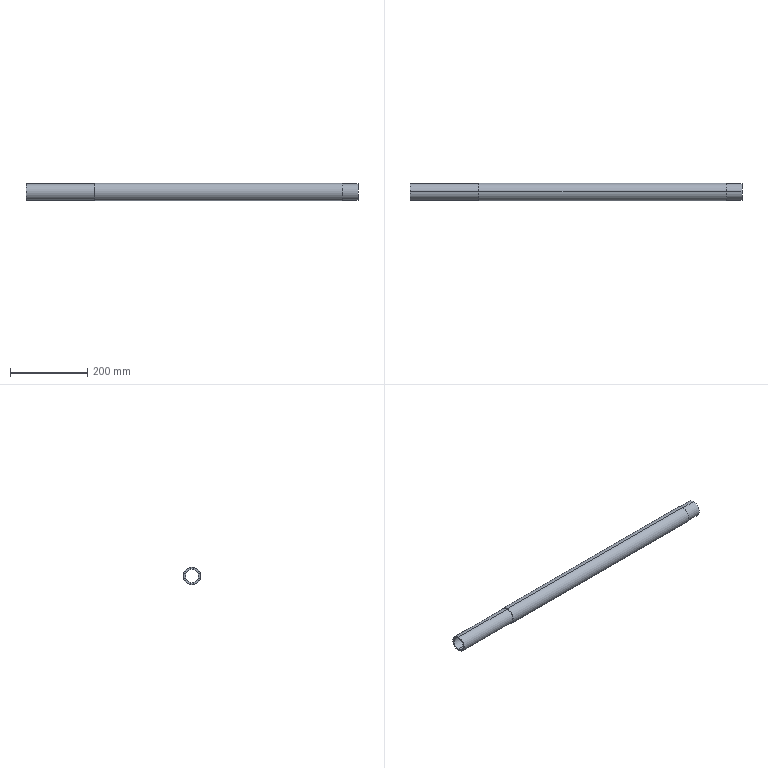Part | SolidWorks | features BaseBody 1 | 1 solid | 12 faces | box 860 x 45 x 45 mm | volume 542272 mm3 | cylinder 8 | plane 4 | commonest cylinder face diameters 42 x4 34 x2 45 x2
STEP:
#1=CARTESIAN_POINT('',(-430.,0.,17.));
#2=VERTEX_POINT('',#1);
#3=CARTESIAN_POINT('',(-430.,0.,-17.));
#4=VERTEX_POINT('',#3);
#5=CARTESIAN_POINT('',(-430.,0.,0.));
#6=DIRECTION('',(1.,0.,0.));
#7=DIRECTION('',(0.,0.,-1.));
#8=AXIS2_PLACEMENT_3D('',#5,#6,#7);
#9=CIRCLE('',#8,17.);
#10=EDGE_CURVE('',#2,#4,#9,.T.);
#11=ORIENTED_EDGE('',*,*,#10,.F.);
#12=CARTESIAN_POINT('',(430.,0.,17.));
#13=VERTEX_POINT('',#12);
#14=CARTESIAN_POINT('',(-473.,0.,17.));
#15=DIRECTION('',(1.,0.,0.));
#16=VECTOR('',#15,1000.);
#17=LINE('',#14,#16);
#18=EDGE_CURVE('',#2,#13,#17,.T.);
#19=ORIENTED_EDGE('',*,*,#18,.T.);
#20=CARTESIAN_POINT('',(430.,0.,-17.));
#21=VERTEX_POINT('',#20);
#22=CARTESIAN_POINT('',(430.,0.,0.));
#23=DIRECTION('',(-1.,0.,0.));
#24=DIRECTION('',(0.,0.,-1.));
#25=AXIS2_PLACEMENT_3D('',#22,#23,#24);
#26=CIRCLE('',#25,17.);
#27=EDGE_CURVE('',#21,#13,#26,.T.);
#28=ORIENTED_EDGE('',*,*,#27,.F.);
#29=CARTESIAN_POINT('',(-473.,0.,-17.));
#30=DIRECTION('',(1.,0.,0.));
#31=VECTOR('',#30,1000.);
#32=LINE('',#29,#31);
#33=EDGE_CURVE('',#4,#21,#32,.T.);
#34=ORIENTED_EDGE('',*,*,#33,.F.);
#35=EDGE_LOOP('',(#11,#19,#28,#34));
#36=FACE_OUTER_BOUND('',#35,.T.);
#37=CARTESIAN_POINT('',(-473.,0.,0.));
#38=DIRECTION('',(1.,0.,0.));
#39=DIRECTION('',(0.,0.,-1.));
#40=AXIS2_PLACEMENT_3D('',#37,#38,#39);
#41=CYLINDRICAL_SURFACE('',#40,17.);
#42=ADVANCED_FACE('',(#36),#41,.F.);
#43=CARTESIAN_POINT('',(390.,0.,-21.));
#44=VERTEX_POINT('',#43);
#45=CARTESIAN_POINT('',(390.,0.,21.));
#46=VERTEX_POINT('',#45);
#47=CARTESIAN_POINT('',(390.,0.,0.));
#48=DIRECTION('',(1.,0.,0.));
#49=DIRECTION('',(0.,0.,-1.));
#50=AXIS2_PLACEMENT_3D('',#47,#48,#49);
#51=CIRCLE('',#50,21.);
#52=EDGE_CURVE('',#44,#46,#51,.T.);
#53=ORIENTED_EDGE('',*,*,#52,.T.);
#54=CARTESIAN_POINT('',(430.,0.,21.));
#55=VERTEX_POINT('',#54);
#56=CARTESIAN_POINT('',(-473.,0.,21.));
#57=DIRECTION('',(1.,0.,0.));
#58=VECTOR('',#57,1000.);
#59=LINE('',#56,#58);
#60=EDGE_CURVE('',#46,#55,#59,.T.);
#61=ORIENTED_EDGE('',*,*,#60,.T.);
#62=CARTESIAN_POINT('',(430.,0.,-21.));
#63=VERTEX_POINT('',#62);
#64=CARTESIAN_POINT('',(430.,0.,0.));
#65=DIRECTION('',(1.,0.,0.));
#66=DIRECTION('',(0.,0.,-1.));
#67=AXIS2_PLACEMENT_3D('',#64,#65,#66);
#68=CIRCLE('',#67,21.);
#69=EDGE_CURVE('',#63,#55,#68,.T.);
#70=ORIENTED_EDGE('',*,*,#69,.F.);
#71=CARTESIAN_POINT('',(-473.,0.,-21.));
#72=DIRECTION('',(1.,0.,0.));
#73=VECTOR('',#72,1000.);
#74=LINE('',#71,#73);
#75=EDGE_CURVE('',#44,#63,#74,.T.);
#76=ORIENTED_EDGE('',*,*,#75,.F.);
#77=EDGE_LOOP('',(#53,#61,#70,#76));
#78=FACE_OUTER_BOUND('',#77,.T.);
#79=CARTESIAN_POINT('',(-473.,0.,0.));
#80=DIRECTION('',(1.,0.,0.));
#81=DIRECTION('',(0.,0.,-1.));
#82=AXIS2_PLACEMENT_3D('',#79,#80,#81);
#83=CYLINDRICAL_SURFACE('',#82,21.);
#84=ADVANCED_FACE('',(#78),#83,.T.);
#85=CARTESIAN_POINT('',(-430.,0.,-21.));
#86=VERTEX_POINT('',#85);
#87=CARTESIAN_POINT('',(-430.,0.,21.));
#88=VERTEX_POINT('',#87);
#89=CARTESIAN_POINT('',(-430.,0.,0.));
#90=DIRECTION('',(1.,0.,0.));
#91=DIRECTION('',(0.,0.,-1.));
#92=AXIS2_PLACEMENT_3D('',#89,#90,#91);
#93=CIRCLE('',#92,21.);
#94=EDGE_CURVE('',#86,#88,#93,.T.);
#95=ORIENTED_EDGE('',*,*,#94,.T.);
#96=CARTESIAN_POINT('',(-252.,0.,21.));
#97=VERTEX_POINT('',#96);
#98=CARTESIAN_POINT('',(-473.,0.,21.));
#99=DIRECTION('',(1.,0.,0.));
#100=VECTOR('',#99,1000.);
#101=LINE('',#98,#100);
#102=EDGE_CURVE('',#88,#97,#101,.T.);
#103=ORIENTED_EDGE('',*,*,#102,.T.);
#104=CARTESIAN_POINT('',(-252.,0.,-21.));
#105=VERTEX_POINT('',#104);
#106=CARTESIAN_POINT('',(-252.,0.,0.));
#107=DIRECTION('',(-1.,0.,0.));
#108=DIRECTION('',(0.,0.,-1.));
#109=AXIS2_PLACEMENT_3D('',#106,#107,#108);
#110=CIRCLE('',#109,21.);
#111=EDGE_CURVE('',#97,#105,#110,.T.);
#112=ORIENTED_EDGE('',*,*,#111,.T.);
#113=CARTESIAN_POINT('',(-473.,0.,-21.));
#114=DIRECTION('',(1.,0.,0.));
#115=VECTOR('',#114,1000.);
#116=LINE('',#113,#115);
#117=EDGE_CURVE('',#86,#105,#116,.T.);
#118=ORIENTED_EDGE('',*,*,#117,.F.);
#119=EDGE_LOOP('',(#95,#103,#112,#118));
#120=FACE_OUTER_BOUND('',#119,.T.);
#121=CARTESIAN_POINT('',(-473.,0.,0.));
#122=DIRECTION('',(1.,0.,0.));
#123=DIRECTION('',(0.,0.,-1.));
#124=AXIS2_PLACEMENT_3D('',#121,#122,#123);
#125=CYLINDRICAL_SURFACE('',#124,21.);
#126=ADVANCED_FACE('',(#120),#125,.T.);
#127=CARTESIAN_POINT('',(-252.,0.,-22.5));
#128=VERTEX_POINT('',#127);
#129=CARTESIAN_POINT('',(-252.,0.,22.5));
#130=VERTEX_POINT('',#129);
#131=CARTESIAN_POINT('',(-252.,0.,0.));
#132=DIRECTION('',(1.,0.,0.));
#133=DIRECTION('',(0.,0.,-1.));
#134=AXIS2_PLACEMENT_3D('',#131,#132,#133);
#135=CIRCLE('',#134,22.5);
#136=EDGE_CURVE('',#128,#130,#135,.T.);
#137=ORIENTED_EDGE('',*,*,#136,.T.);
#138=CARTESIAN_POINT('',(390.,0.,22.5));
#139=VERTEX_POINT('',#138);
#140=CARTESIAN_POINT('',(-473.,0.,22.5));
#141=DIRECTION('',(1.,0.,0.));
#142=VECTOR('',#141,1000.);
#143=LINE('',#140,#142);
#144=EDGE_CURVE('',#130,#139,#143,.T.);
#145=ORIENTED_EDGE('',*,*,#144,.T.);
#146=CARTESIAN_POINT('',(390.,0.,-22.5));
#147=VERTEX_POINT('',#146);
#148=CARTESIAN_POINT('',(390.,0.,0.));
#149=DIRECTION('',(1.,0.,0.));
#150=DIRECTION('',(0.,0.,-1.));
#151=AXIS2_PLACEMENT_3D('',#148,#149,#150);
#152=CIRCLE('',#151,22.5);
#153=EDGE_CURVE('',#147,#139,#152,.T.);
#154=ORIENTED_EDGE('',*,*,#153,.F.);
#155=CARTESIAN_POINT('',(-473.,0.,-22.5));
#156=DIRECTION('',(1.,0.,0.));
#157=VECTOR('',#156,1000.);
#158=LINE('',#155,#157);
#159=EDGE_CURVE('',#128,#147,#158,.T.);
#160=ORIENTED_EDGE('',*,*,#159,.F.);
#161=EDGE_LOOP('',(#137,#145,#154,#160));
#162=FACE_OUTER_BOUND('',#161,.T.);
#163=CARTESIAN_POINT('',(-473.,0.,0.));
#164=DIRECTION('',(1.,0.,0.));
#165=DIRECTION('',(0.,0.,-1.));
#166=AXIS2_PLACEMENT_3D('',#163,#164,#165);
#167=CYLINDRICAL_SURFACE('',#166,22.5);
#168=ADVANCED_FACE('',(#162),#167,.T.);
#169=ORIENTED_EDGE('',*,*,#18,.F.);
#170=CARTESIAN_POINT('',(-430.,0.,0.));
#171=DIRECTION('',(1.,0.,0.));
#172=DIRECTION('',(0.,0.,-1.));
#173=AXIS2_PLACEMENT_3D('',#170,#171,#172);
#174=CIRCLE('',#173,17.);
#175=EDGE_CURVE('',#4,#2,#174,.T.);
#176=ORIENTED_EDGE('',*,*,#175,.F.);
#177=ORIENTED_EDGE('',*,*,#33,.T.);
#178=CARTESIAN_POINT('',(430.,0.,0.));
#179=DIRECTION('',(-1.,0.,0.));
#180=DIRECTION('',(0.,0.,-1.));
#181=AXIS2_PLACEMENT_3D('',#178,#179,#180);
#182=CIRCLE('',#181,17.);
#183=EDGE_CURVE('',#13,#21,#182,.T.);
#184=ORIENTED_EDGE('',*,*,#183,.F.);
#185=EDGE_LOOP('',(#169,#176,#177,#184));
#186=FACE_OUTER_BOUND('',#185,.T.);
#187=CARTESIAN_POINT('',(-473.,0.,0.));
#188=DIRECTION('',(1.,0.,0.));
#189=DIRECTION('',(0.,0.,-1.));
#190=AXIS2_PLACEMENT_3D('',#187,#188,#189);
#191=CYLINDRICAL_SURFACE('',#190,17.);
#192=ADVANCED_FACE('',(#186),#191,.F.);
#193=ORIENTED_EDGE('',*,*,#27,.T.);
#194=ORIENTED_EDGE('',*,*,#183,.T.);
#195=EDGE_LOOP('',(#193,#194));
#196=FACE_BOUND('',#195,.T.);
#197=ORIENTED_EDGE('',*,*,#69,.T.);
#198=CARTESIAN_POINT('',(430.,0.,0.));
#199=DIRECTION('',(1.,0.,0.));
#200=DIRECTION('',(0.,0.,-1.));
#201=AXIS2_PLACEMENT_3D('',#198,#199,#200);
#202=CIRCLE('',#201,21.);
#203=EDGE_CURVE('',#55,#63,#202,.T.);
#204=ORIENTED_EDGE('',*,*,#203,.T.);
#205=EDGE_LOOP('',(#197,#204));
#206=FACE_OUTER_BOUND('',#205,.T.);
#207=CARTESIAN_POINT('',(430.,0.,0.));
#208=DIRECTION('',(1.,0.,0.));
#209=DIRECTION('',(0.,0.,-1.));
#210=AXIS2_PLACEMENT_3D('',#207,#208,#209);
#211=PLANE('',#210);
#212=ADVANCED_FACE('',(#196,#206),#211,.T.);
#213=ORIENTED_EDGE('',*,*,#175,.T.);
#214=ORIENTED_EDGE('',*,*,#10,.T.);
#215=EDGE_LOOP('',(#213,#214));
#216=FACE_BOUND('',#215,.T.);
#217=ORIENTED_EDGE('',*,*,#94,.F.);
#218=CARTESIAN_POINT('',(-430.,0.,0.));
#219=DIRECTION('',(1.,0.,0.));
#220=DIRECTION('',(0.,0.,-1.));
#221=AXIS2_PLACEMENT_3D('',#218,#219,#220);
#222=CIRCLE('',#221,21.);
#223=EDGE_CURVE('',#88,#86,#222,.T.);
#224=ORIENTED_EDGE('',*,*,#223,.F.);
#225=EDGE_LOOP('',(#217,#224));
#226=FACE_OUTER_BOUND('',#225,.T.);
#227=CARTESIAN_POINT('',(-430.,0.,0.));
#228=DIRECTION('',(1.,0.,0.));
#229=DIRECTION('',(0.,0.,-1.));
#230=AXIS2_PLACEMENT_3D('',#227,#228,#229);
#231=PLANE('',#230);
#232=ADVANCED_FACE('',(#216,#226),#231,.F.);
#233=ORIENTED_EDGE('',*,*,#60,.F.);
#234=CARTESIAN_POINT('',(390.,0.,0.));
#235=DIRECTION('',(1.,0.,0.));
#236=DIRECTION('',(0.,0.,-1.));
#237=AXIS2_PLACEMENT_3D('',#234,#235,#236);
#238=CIRCLE('',#237,21.);
#239=EDGE_CURVE('',#46,#44,#238,.T.);
#240=ORIENTED_EDGE('',*,*,#239,.T.);
#241=ORIENTED_EDGE('',*,*,#75,.T.);
#242=ORIENTED_EDGE('',*,*,#203,.F.);
#243=EDGE_LOOP('',(#233,#240,#241,#242));
#244=FACE_OUTER_BOUND('',#243,.T.);
#245=CARTESIAN_POINT('',(-473.,0.,0.));
#246=DIRECTION('',(1.,0.,0.));
#247=DIRECTION('',(0.,0.,-1.));
#248=AXIS2_PLACEMENT_3D('',#245,#246,#247);
#249=CYLINDRICAL_SURFACE('',#248,21.);
#250=ADVANCED_FACE('',(#244),#249,.T.);
#251=ORIENTED_EDGE('',*,*,#102,.F.);
#252=ORIENTED_EDGE('',*,*,#223,.T.);
#253=ORIENTED_EDGE('',*,*,#117,.T.);
#254=CARTESIAN_POINT('',(-252.,0.,0.));
#255=DIRECTION('',(-1.,0.,0.));
#256=DIRECTION('',(0.,0.,-1.));
#257=AXIS2_PLACEMENT_3D('',#254,#255,#256);
#258=CIRCLE('',#257,21.);
#259=EDGE_CURVE('',#105,#97,#258,.T.);
#260=ORIENTED_EDGE('',*,*,#259,.T.);
#261=EDGE_LOOP('',(#251,#252,#253,#260));
#262=FACE_OUTER_BOUND('',#261,.T.);
#263=CARTESIAN_POINT('',(-473.,0.,0.));
#264=DIRECTION('',(1.,0.,0.));
#265=DIRECTION('',(0.,0.,-1.));
#266=AXIS2_PLACEMENT_3D('',#263,#264,#265);
#267=CYLINDRICAL_SURFACE('',#266,21.);
#268=ADVANCED_FACE('',(#262),#267,.T.);
#269=ORIENTED_EDGE('',*,*,#52,.F.);
#270=ORIENTED_EDGE('',*,*,#239,.F.);
#271=EDGE_LOOP('',(#269,#270));
#272=FACE_BOUND('',#271,.T.);
#273=ORIENTED_EDGE('',*,*,#153,.T.);
#274=CARTESIAN_POINT('',(390.,0.,0.));
#275=DIRECTION('',(1.,0.,0.));
#276=DIRECTION('',(0.,0.,-1.));
#277=AXIS2_PLACEMENT_3D('',#274,#275,#276);
#278=CIRCLE('',#277,22.5);
#279=EDGE_CURVE('',#139,#147,#278,.T.);
#280=ORIENTED_EDGE('',*,*,#279,.T.);
#281=EDGE_LOOP('',(#273,#280));
#282=FACE_OUTER_BOUND('',#281,.T.);
#283=CARTESIAN_POINT('',(390.,0.,0.));
#284=DIRECTION('',(1.,0.,0.));
#285=DIRECTION('',(0.,0.,-1.));
#286=AXIS2_PLACEMENT_3D('',#283,#284,#285);
#287=PLANE('',#286);
#288=ADVANCED_FACE('',(#272,#282),#287,.T.);
#289=ORIENTED_EDGE('',*,*,#259,.F.);
#290=ORIENTED_EDGE('',*,*,#111,.F.);
#291=EDGE_LOOP('',(#289,#290));
#292=FACE_BOUND('',#291,.T.);
#293=ORIENTED_EDGE('',*,*,#136,.F.);
#294=CARTESIAN_POINT('',(-252.,0.,0.));
#295=DIRECTION('',(1.,0.,0.));
#296=DIRECTION('',(0.,0.,-1.));
#297=AXIS2_PLACEMENT_3D('',#294,#295,#296);
#298=CIRCLE('',#297,22.5);
#299=EDGE_CURVE('',#130,#128,#298,.T.);
#300=ORIENTED_EDGE('',*,*,#299,.F.);
#301=EDGE_LOOP('',(#293,#300));
#302=FACE_OUTER_BOUND('',#301,.T.);
#303=CARTESIAN_POINT('',(-252.,0.,0.));
#304=DIRECTION('',(1.,0.,0.));
#305=DIRECTION('',(0.,0.,-1.));
#306=AXIS2_PLACEMENT_3D('',#303,#304,#305);
#307=PLANE('',#306);
#308=ADVANCED_FACE('',(#292,#302),#307,.F.);
#309=ORIENTED_EDGE('',*,*,#144,.F.);
#310=ORIENTED_EDGE('',*,*,#299,.T.);
#311=ORIENTED_EDGE('',*,*,#159,.T.);
#312=ORIENTED_EDGE('',*,*,#279,.F.);
#313=EDGE_LOOP('',(#309,#310,#311,#312));
#314=FACE_OUTER_BOUND('',#313,.T.);
#315=CARTESIAN_POINT('',(-473.,0.,0.));
#316=DIRECTION('',(1.,0.,0.));
#317=DIRECTION('',(0.,0.,-1.));
#318=AXIS2_PLACEMENT_3D('',#315,#316,#317);
#319=CYLINDRICAL_SURFACE('',#318,22.5);
#320=ADVANCED_FACE('',(#314),#319,.T.);
#321=CLOSED_SHELL('',(#42,#84,#126,#168,#192,#212,#232,#250,#268,#288,#308,#320));
#322=MANIFOLD_SOLID_BREP('',#321);
#323=CARTESIAN_POINT('',(0.,0.,0.));
#324=DIRECTION('',(0.,0.,1.));
#325=DIRECTION('',(1.,0.,0.));
#326=AXIS2_PLACEMENT_3D('',#323,#324,#325);
#327=(LENGTH_UNIT()NAMED_UNIT(*)SI_UNIT(.MILLI.,.METRE.));
#328=UNCERTAINTY_MEASURE_WITH_UNIT(LENGTH_MEASURE(0.00001),#327,'','');
#329=(NAMED_UNIT(*)PLANE_ANGLE_UNIT()SI_UNIT($,.RADIAN.));
#330=(NAMED_UNIT(*)SI_UNIT($,.STERADIAN.)SOLID_ANGLE_UNIT());
#331=(GEOMETRIC_REPRESENTATION_CONTEXT(3)GLOBAL_UNCERTAINTY_ASSIGNED_CONTEXT((#328))GLOBAL_UNIT_ASSIGNED_CONTEXT((#327,#329,#330))REPRESENTATION_CONTEXT('',''));
#332=ADVANCED_BREP_SHAPE_REPRESENTATION('',(#322,#326),#331);